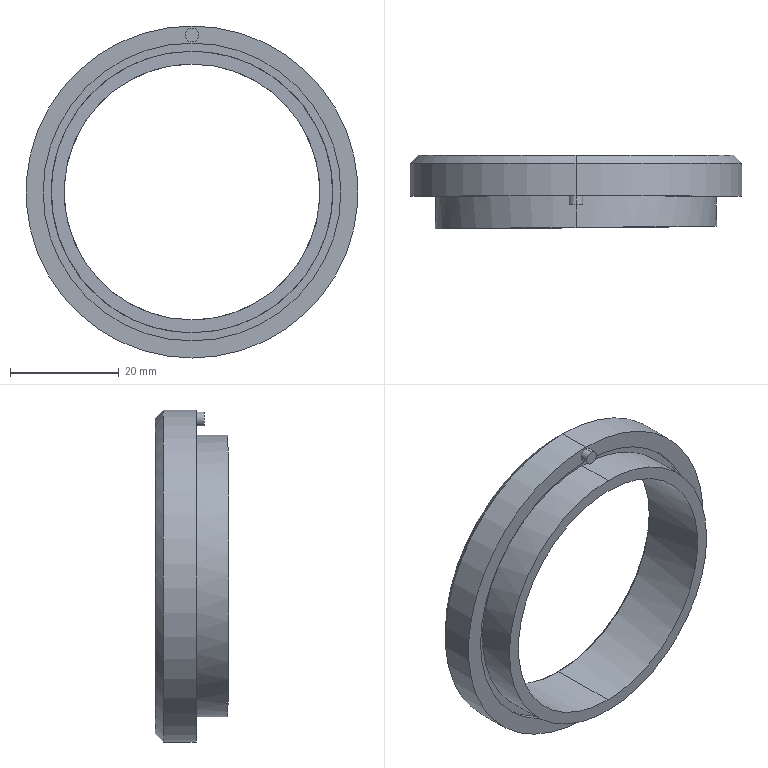Part | SolidWorks | features Chamfer 2, ICE 2, Revolution 1 | 1 solid | 19 faces | box 61 x 13.5 x 61 mm | volume 10536 mm3 | cylinder 10 | plane 5 | cone 4 | commonest cylinder face diameters 2.5 x2 47 x2 51.7 x2 54.7 x2 61 x2
STEP:
#1=CARTESIAN_POINT('',(0.,-1.5,27.6));
#2=VERTEX_POINT('',#1);
#3=CARTESIAN_POINT('',(0.,-1.5,30.1));
#4=VERTEX_POINT('',#3);
#5=CARTESIAN_POINT('',(0.,-1.5,28.85));
#6=DIRECTION('',(0.,-1.,0.));
#7=DIRECTION('',(0.,0.,-1.));
#8=AXIS2_PLACEMENT_3D('',#5,#6,#7);
#9=CIRCLE('',#8,1.25);
#10=EDGE_CURVE('',#2,#4,#9,.T.);
#11=ORIENTED_EDGE('',*,*,#10,.F.);
#12=CARTESIAN_POINT('',(0.,0.,27.6));
#13=VERTEX_POINT('',#12);
#14=CARTESIAN_POINT('',(0.,-1.5,27.6));
#15=DIRECTION('',(0.,1.,0.));
#16=VECTOR('',#15,1000.);
#17=LINE('',#14,#16);
#18=EDGE_CURVE('',#2,#13,#17,.T.);
#19=ORIENTED_EDGE('',*,*,#18,.T.);
#20=CARTESIAN_POINT('',(0.,0.,30.1));
#21=VERTEX_POINT('',#20);
#22=CARTESIAN_POINT('',(0.,0.,28.85));
#23=DIRECTION('',(0.,-1.,0.));
#24=DIRECTION('',(0.,0.,-1.));
#25=AXIS2_PLACEMENT_3D('',#22,#23,#24);
#26=CIRCLE('',#25,1.25);
#27=EDGE_CURVE('',#13,#21,#26,.T.);
#28=ORIENTED_EDGE('',*,*,#27,.T.);
#29=CARTESIAN_POINT('',(0.,-1.5,30.1));
#30=DIRECTION('',(0.,1.,0.));
#31=VECTOR('',#30,1000.);
#32=LINE('',#29,#31);
#33=EDGE_CURVE('',#4,#21,#32,.T.);
#34=ORIENTED_EDGE('',*,*,#33,.F.);
#35=EDGE_LOOP('',(#11,#19,#28,#34));
#36=FACE_OUTER_BOUND('',#35,.T.);
#37=CARTESIAN_POINT('',(0.,-1.5,28.85));
#38=DIRECTION('',(0.,1.,0.));
#39=DIRECTION('',(0.,0.,1.));
#40=AXIS2_PLACEMENT_3D('',#37,#38,#39);
#41=CYLINDRICAL_SURFACE('',#40,1.25);
#42=ADVANCED_FACE('',(#36),#41,.T.);
#43=CARTESIAN_POINT('',(0.,7.5,29.));
#44=VERTEX_POINT('',#43);
#45=CARTESIAN_POINT('',(0.,7.5,-29.));
#46=VERTEX_POINT('',#45);
#47=CARTESIAN_POINT('',(0.,7.5,0.));
#48=DIRECTION('',(0.,1.,0.));
#49=DIRECTION('',(0.,0.,1.));
#50=AXIS2_PLACEMENT_3D('',#47,#48,#49);
#51=CIRCLE('',#50,29.);
#52=EDGE_CURVE('',#44,#46,#51,.T.);
#53=ORIENTED_EDGE('',*,*,#52,.F.);
#54=CARTESIAN_POINT('',(0.,6.,30.5));
#55=VERTEX_POINT('',#54);
#56=CARTESIAN_POINT('',(0.,6.,30.5));
#57=DIRECTION('',(0.,-0.7071,0.7071));
#58=VECTOR('',#57,1000.);
#59=LINE('',#56,#58);
#60=EDGE_CURVE('',#44,#55,#59,.T.);
#61=ORIENTED_EDGE('',*,*,#60,.T.);
#62=CARTESIAN_POINT('',(0.,6.,-30.5));
#63=VERTEX_POINT('',#62);
#64=CARTESIAN_POINT('',(0.,6.,0.));
#65=DIRECTION('',(0.,-1.,0.));
#66=DIRECTION('',(0.,0.,1.));
#67=AXIS2_PLACEMENT_3D('',#64,#65,#66);
#68=CIRCLE('',#67,30.5);
#69=EDGE_CURVE('',#63,#55,#68,.T.);
#70=ORIENTED_EDGE('',*,*,#69,.F.);
#71=CARTESIAN_POINT('',(0.,6.,-30.5));
#72=DIRECTION('',(0.,-0.7071,-0.7071));
#73=VECTOR('',#72,1000.);
#74=LINE('',#71,#73);
#75=EDGE_CURVE('',#46,#63,#74,.T.);
#76=ORIENTED_EDGE('',*,*,#75,.F.);
#77=EDGE_LOOP('',(#53,#61,#70,#76));
#78=FACE_OUTER_BOUND('',#77,.T.);
#79=CARTESIAN_POINT('',(0.,6.,0.));
#80=DIRECTION('',(0.,-1.,0.));
#81=DIRECTION('',(0.,0.,-1.));
#82=AXIS2_PLACEMENT_3D('',#79,#80,#81);
#83=CONICAL_SURFACE('',#82,30.5,0.7854);
#84=ADVANCED_FACE('',(#78),#83,.T.);
#85=CARTESIAN_POINT('',(0.,7.,-23.5));
#86=VERTEX_POINT('',#85);
#87=CARTESIAN_POINT('',(0.,7.,23.5));
#88=VERTEX_POINT('',#87);
#89=CARTESIAN_POINT('',(0.,7.,0.));
#90=DIRECTION('',(0.,1.,0.));
#91=DIRECTION('',(0.,0.,1.));
#92=AXIS2_PLACEMENT_3D('',#89,#90,#91);
#93=CIRCLE('',#92,23.5);
#94=EDGE_CURVE('',#86,#88,#93,.T.);
#95=ORIENTED_EDGE('',*,*,#94,.F.);
#96=CARTESIAN_POINT('',(0.,7.5,-24.));
#97=VERTEX_POINT('',#96);
#98=CARTESIAN_POINT('',(0.,7.5,-24.));
#99=DIRECTION('',(0.,0.7071,-0.7071));
#100=VECTOR('',#99,1000.);
#101=LINE('',#98,#100);
#102=EDGE_CURVE('',#86,#97,#101,.T.);
#103=ORIENTED_EDGE('',*,*,#102,.T.);
#104=CARTESIAN_POINT('',(0.,7.5,24.));
#105=VERTEX_POINT('',#104);
#106=CARTESIAN_POINT('',(0.,7.5,0.));
#107=DIRECTION('',(0.,-1.,0.));
#108=DIRECTION('',(0.,0.,1.));
#109=AXIS2_PLACEMENT_3D('',#106,#107,#108);
#110=CIRCLE('',#109,24.);
#111=EDGE_CURVE('',#105,#97,#110,.T.);
#112=ORIENTED_EDGE('',*,*,#111,.F.);
#113=CARTESIAN_POINT('',(0.,7.5,24.));
#114=DIRECTION('',(0.,0.7071,0.7071));
#115=VECTOR('',#114,1000.);
#116=LINE('',#113,#115);
#117=EDGE_CURVE('',#88,#105,#116,.T.);
#118=ORIENTED_EDGE('',*,*,#117,.F.);
#119=EDGE_LOOP('',(#95,#103,#112,#118));
#120=FACE_OUTER_BOUND('',#119,.T.);
#121=CARTESIAN_POINT('',(0.,7.5,0.));
#122=DIRECTION('',(0.,1.,0.));
#123=DIRECTION('',(0.,0.,1.));
#124=AXIS2_PLACEMENT_3D('',#121,#122,#123);
#125=CONICAL_SURFACE('',#124,24.,0.7854);
#126=ADVANCED_FACE('',(#120),#125,.F.);
#127=CARTESIAN_POINT('',(0.,1.,-25.85));
#128=VERTEX_POINT('',#127);
#129=CARTESIAN_POINT('',(0.,1.,25.85));
#130=VERTEX_POINT('',#129);
#131=CARTESIAN_POINT('',(0.,1.,0.));
#132=DIRECTION('',(0.,-1.,0.));
#133=DIRECTION('',(0.,0.,-1.));
#134=AXIS2_PLACEMENT_3D('',#131,#132,#133);
#135=CIRCLE('',#134,25.85);
#136=EDGE_CURVE('',#128,#130,#135,.T.);
#137=ORIENTED_EDGE('',*,*,#136,.T.);
#138=CARTESIAN_POINT('',(0.,-5.774,25.85));
#139=VERTEX_POINT('',#138);
#140=CARTESIAN_POINT('',(0.,0.,25.85));
#141=DIRECTION('',(0.,-1.,0.));
#142=VECTOR('',#141,1000.);
#143=LINE('',#140,#142);
#144=EDGE_CURVE('',#130,#139,#143,.T.);
#145=ORIENTED_EDGE('',*,*,#144,.T.);
#146=CARTESIAN_POINT('',(0.,-5.774,-25.85));
#147=VERTEX_POINT('',#146);
#148=CARTESIAN_POINT('',(0.,-5.774,-25.85));
#149=CARTESIAN_POINT('',(51.7,-5.323,-25.85));
#150=CARTESIAN_POINT('',(51.7,-5.323,25.85));
#151=CARTESIAN_POINT('',(0.,-5.774,25.85));
#152=(BOUNDED_CURVE()B_SPLINE_CURVE(3,(#148,#149,#150,#151),.UNSPECIFIED.,.F.,.F.)B_SPLINE_CURVE_WITH_KNOTS((4,4),(1.571,4.712),.UNSPECIFIED.)CURVE()GEOMETRIC_REPRESENTATION_ITEM()RATIONAL_B_SPLINE_CURVE((1.,0.3333,0.3333,1.))REPRESENTATION_ITEM(''));
#153=EDGE_CURVE('',#147,#139,#152,.T.);
#154=ORIENTED_EDGE('',*,*,#153,.F.);
#155=CARTESIAN_POINT('',(0.,0.,-25.85));
#156=DIRECTION('',(0.,-1.,0.));
#157=VECTOR('',#156,1000.);
#158=LINE('',#155,#157);
#159=EDGE_CURVE('',#128,#147,#158,.T.);
#160=ORIENTED_EDGE('',*,*,#159,.F.);
#161=EDGE_LOOP('',(#137,#145,#154,#160));
#162=FACE_OUTER_BOUND('',#161,.T.);
#163=CARTESIAN_POINT('',(0.,0.,0.));
#164=DIRECTION('',(0.,-1.,0.));
#165=DIRECTION('',(0.,0.,-1.));
#166=AXIS2_PLACEMENT_3D('',#163,#164,#165);
#167=CYLINDRICAL_SURFACE('',#166,25.85);
#168=ADVANCED_FACE('',(#162),#167,.T.);
#169=CARTESIAN_POINT('',(0.,1.,27.35));
#170=VERTEX_POINT('',#169);
#171=CARTESIAN_POINT('',(0.,1.,-27.35));
#172=VERTEX_POINT('',#171);
#173=CARTESIAN_POINT('',(0.,1.,0.));
#174=DIRECTION('',(0.,-1.,0.));
#175=DIRECTION('',(0.,0.,-1.));
#176=AXIS2_PLACEMENT_3D('',#173,#174,#175);
#177=CIRCLE('',#176,27.35);
#178=EDGE_CURVE('',#170,#172,#177,.T.);
#179=ORIENTED_EDGE('',*,*,#178,.F.);
#180=CARTESIAN_POINT('',(0.,0.,27.35));
#181=VERTEX_POINT('',#180);
#182=CARTESIAN_POINT('',(0.,0.,27.35));
#183=DIRECTION('',(0.,-1.,0.));
#184=VECTOR('',#183,1000.);
#185=LINE('',#182,#184);
#186=EDGE_CURVE('',#170,#181,#185,.T.);
#187=ORIENTED_EDGE('',*,*,#186,.T.);
#188=CARTESIAN_POINT('',(0.,0.,-27.35));
#189=VERTEX_POINT('',#188);
#190=CARTESIAN_POINT('',(0.,0.,0.));
#191=DIRECTION('',(0.,-1.,0.));
#192=DIRECTION('',(0.,0.,-1.));
#193=AXIS2_PLACEMENT_3D('',#190,#191,#192);
#194=CIRCLE('',#193,27.35);
#195=EDGE_CURVE('',#181,#189,#194,.T.);
#196=ORIENTED_EDGE('',*,*,#195,.T.);
#197=CARTESIAN_POINT('',(0.,0.,-27.35));
#198=DIRECTION('',(0.,-1.,0.));
#199=VECTOR('',#198,1000.);
#200=LINE('',#197,#199);
#201=EDGE_CURVE('',#172,#189,#200,.T.);
#202=ORIENTED_EDGE('',*,*,#201,.F.);
#203=EDGE_LOOP('',(#179,#187,#196,#202));
#204=FACE_OUTER_BOUND('',#203,.T.);
#205=CARTESIAN_POINT('',(0.,0.,0.));
#206=DIRECTION('',(0.,-1.,0.));
#207=DIRECTION('',(0.,0.,-1.));
#208=AXIS2_PLACEMENT_3D('',#205,#206,#207);
#209=CYLINDRICAL_SURFACE('',#208,27.35);
#210=ADVANCED_FACE('',(#204),#209,.F.);
#211=ORIENTED_EDGE('',*,*,#69,.T.);
#212=CARTESIAN_POINT('',(0.,0.,30.5));
#213=VERTEX_POINT('',#212);
#214=CARTESIAN_POINT('',(0.,0.,30.5));
#215=DIRECTION('',(0.,-1.,0.));
#216=VECTOR('',#215,1000.);
#217=LINE('',#214,#216);
#218=EDGE_CURVE('',#55,#213,#217,.T.);
#219=ORIENTED_EDGE('',*,*,#218,.T.);
#220=CARTESIAN_POINT('',(0.,0.,-30.5));
#221=VERTEX_POINT('',#220);
#222=CARTESIAN_POINT('',(0.,0.,0.));
#223=DIRECTION('',(0.,-1.,0.));
#224=DIRECTION('',(0.,0.,-1.));
#225=AXIS2_PLACEMENT_3D('',#222,#223,#224);
#226=CIRCLE('',#225,30.5);
#227=EDGE_CURVE('',#221,#213,#226,.T.);
#228=ORIENTED_EDGE('',*,*,#227,.F.);
#229=CARTESIAN_POINT('',(0.,0.,-30.5));
#230=DIRECTION('',(0.,-1.,0.));
#231=VECTOR('',#230,1000.);
#232=LINE('',#229,#231);
#233=EDGE_CURVE('',#63,#221,#232,.T.);
#234=ORIENTED_EDGE('',*,*,#233,.F.);
#235=EDGE_LOOP('',(#211,#219,#228,#234));
#236=FACE_OUTER_BOUND('',#235,.T.);
#237=CARTESIAN_POINT('',(0.,0.,0.));
#238=DIRECTION('',(0.,-1.,0.));
#239=DIRECTION('',(0.,0.,-1.));
#240=AXIS2_PLACEMENT_3D('',#237,#238,#239);
#241=CYLINDRICAL_SURFACE('',#240,30.5);
#242=ADVANCED_FACE('',(#236),#241,.T.);
#243=ORIENTED_EDGE('',*,*,#94,.T.);
#244=CARTESIAN_POINT('',(0.,-5.774,23.5));
#245=VERTEX_POINT('',#244);
#246=CARTESIAN_POINT('',(0.,0.,23.5));
#247=DIRECTION('',(0.,-1.,0.));
#248=VECTOR('',#247,1000.);
#249=LINE('',#246,#248);
#250=EDGE_CURVE('',#88,#245,#249,.T.);
#251=ORIENTED_EDGE('',*,*,#250,.T.);
#252=CARTESIAN_POINT('',(0.,-5.774,-23.5));
#253=VERTEX_POINT('',#252);
#254=CARTESIAN_POINT('',(0.,-5.774,-23.5));
#255=CARTESIAN_POINT('',(-47.,-6.185,-23.5));
#256=CARTESIAN_POINT('',(-47.,-6.185,23.5));
#257=CARTESIAN_POINT('',(0.,-5.774,23.5));
#258=(BOUNDED_CURVE()B_SPLINE_CURVE(3,(#254,#255,#256,#257),.UNSPECIFIED.,.F.,.F.)B_SPLINE_CURVE_WITH_KNOTS((4,4),(4.712,7.854),.UNSPECIFIED.)CURVE()GEOMETRIC_REPRESENTATION_ITEM()RATIONAL_B_SPLINE_CURVE((1.,0.3333,0.3333,1.))REPRESENTATION_ITEM(''));
#259=EDGE_CURVE('',#253,#245,#258,.T.);
#260=ORIENTED_EDGE('',*,*,#259,.F.);
#261=CARTESIAN_POINT('',(0.,0.,-23.5));
#262=DIRECTION('',(0.,-1.,0.));
#263=VECTOR('',#262,1000.);
#264=LINE('',#261,#263);
#265=EDGE_CURVE('',#86,#253,#264,.T.);
#266=ORIENTED_EDGE('',*,*,#265,.F.);
#267=EDGE_LOOP('',(#243,#251,#260,#266));
#268=FACE_OUTER_BOUND('',#267,.T.);
#269=CARTESIAN_POINT('',(0.,0.,0.));
#270=DIRECTION('',(0.,-1.,0.));
#271=DIRECTION('',(0.,0.,-1.));
#272=AXIS2_PLACEMENT_3D('',#269,#270,#271);
#273=CYLINDRICAL_SURFACE('',#272,23.5);
#274=ADVANCED_FACE('',(#268),#273,.F.);
#275=ORIENTED_EDGE('',*,*,#250,.F.);
#276=CARTESIAN_POINT('',(0.,7.,0.));
#277=DIRECTION('',(0.,1.,0.));
#278=DIRECTION('',(0.,0.,1.));
#279=AXIS2_PLACEMENT_3D('',#276,#277,#278);
#280=CIRCLE('',#279,23.5);
#281=EDGE_CURVE('',#88,#86,#280,.T.);
#282=ORIENTED_EDGE('',*,*,#281,.T.);
#283=ORIENTED_EDGE('',*,*,#265,.T.);
#284=CARTESIAN_POINT('',(0.,-5.774,23.5));
#285=CARTESIAN_POINT('',(47.,-5.364,23.5));
#286=CARTESIAN_POINT('',(47.,-5.364,-23.5));
#287=CARTESIAN_POINT('',(0.,-5.774,-23.5));
#288=(BOUNDED_CURVE()B_SPLINE_CURVE(3,(#284,#285,#286,#287),.UNSPECIFIED.,.F.,.F.)B_SPLINE_CURVE_WITH_KNOTS((4,4),(1.571,4.712),.UNSPECIFIED.)CURVE()GEOMETRIC_REPRESENTATION_ITEM()RATIONAL_B_SPLINE_CURVE((1.,0.3333,0.3333,1.))REPRESENTATION_ITEM(''));
#289=EDGE_CURVE('',#245,#253,#288,.T.);
#290=ORIENTED_EDGE('',*,*,#289,.F.);
#291=EDGE_LOOP('',(#275,#282,#283,#290));
#292=FACE_OUTER_BOUND('',#291,.T.);
#293=CARTESIAN_POINT('',(0.,0.,0.));
#294=DIRECTION('',(0.,-1.,0.));
#295=DIRECTION('',(0.,0.,-1.));
#296=AXIS2_PLACEMENT_3D('',#293,#294,#295);
#297=CYLINDRICAL_SURFACE('',#296,23.5);
#298=ADVANCED_FACE('',(#292),#297,.F.);
#299=CARTESIAN_POINT('',(0.,7.5,0.));
#300=DIRECTION('',(0.,1.,0.));
#301=DIRECTION('',(0.,0.,1.));
#302=AXIS2_PLACEMENT_3D('',#299,#300,#301);
#303=CIRCLE('',#302,29.);
#304=EDGE_CURVE('',#46,#44,#303,.T.);
#305=ORIENTED_EDGE('',*,*,#304,.T.);
#306=ORIENTED_EDGE('',*,*,#52,.T.);
#307=EDGE_LOOP('',(#305,#306));
#308=FACE_OUTER_BOUND('',#307,.T.);
#309=ORIENTED_EDGE('',*,*,#111,.T.);
#310=CARTESIAN_POINT('',(0.,7.5,0.));
#311=DIRECTION('',(0.,-1.,0.));
#312=DIRECTION('',(0.,0.,1.));
#313=AXIS2_PLACEMENT_3D('',#310,#311,#312);
#314=CIRCLE('',#313,24.);
#315=EDGE_CURVE('',#97,#105,#314,.T.);
#316=ORIENTED_EDGE('',*,*,#315,.T.);
#317=EDGE_LOOP('',(#309,#316));
#318=FACE_BOUND('',#317,.T.);
#319=CARTESIAN_POINT('',(30.5,7.5,0.));
#320=DIRECTION('',(0.,1.,0.));
#321=DIRECTION('',(0.,0.,1.));
#322=AXIS2_PLACEMENT_3D('',#319,#320,#321);
#323=PLANE('',#322);
#324=ADVANCED_FACE('',(#308,#318),#323,.T.);
#325=ORIENTED_EDGE('',*,*,#218,.F.);
#326=CARTESIAN_POINT('',(0.,6.,0.));
#327=DIRECTION('',(0.,-1.,0.));
#328=DIRECTION('',(0.,0.,1.));
#329=AXIS2_PLACEMENT_3D('',#326,#327,#328);
#330=CIRCLE('',#329,30.5);
#331=EDGE_CURVE('',#55,#63,#330,.T.);
#332=ORIENTED_EDGE('',*,*,#331,.T.);
#333=ORIENTED_EDGE('',*,*,#233,.T.);
#334=CARTESIAN_POINT('',(0.,0.,0.));
#335=DIRECTION('',(0.,-1.,0.));
#336=DIRECTION('',(0.,0.,-1.));
#337=AXIS2_PLACEMENT_3D('',#334,#335,#336);
#338=CIRCLE('',#337,30.5);
#339=EDGE_CURVE('',#213,#221,#338,.T.);
#340=ORIENTED_EDGE('',*,*,#339,.F.);
#341=EDGE_LOOP('',(#325,#332,#333,#340));
#342=FACE_OUTER_BOUND('',#341,.T.);
#343=CARTESIAN_POINT('',(0.,0.,0.));
#344=DIRECTION('',(0.,-1.,0.));
#345=DIRECTION('',(0.,0.,-1.));
#346=AXIS2_PLACEMENT_3D('',#343,#344,#345);
#347=CYLINDRICAL_SURFACE('',#346,30.5);
#348=ADVANCED_FACE('',(#342),#347,.T.);
#349=CARTESIAN_POINT('',(0.,0.,28.85));
#350=DIRECTION('',(0.,-1.,0.));
#351=DIRECTION('',(0.,0.,-1.));
#352=AXIS2_PLACEMENT_3D('',#349,#350,#351);
#353=CIRCLE('',#352,1.25);
#354=EDGE_CURVE('',#21,#13,#353,.T.);
#355=ORIENTED_EDGE('',*,*,#354,.F.);
#356=ORIENTED_EDGE('',*,*,#27,.F.);
#357=EDGE_LOOP('',(#355,#356));
#358=FACE_BOUND('',#357,.T.);
#359=ORIENTED_EDGE('',*,*,#227,.T.);
#360=ORIENTED_EDGE('',*,*,#339,.T.);
#361=EDGE_LOOP('',(#359,#360));
#362=FACE_OUTER_BOUND('',#361,.T.);
#363=CARTESIAN_POINT('',(0.,0.,0.));
#364=DIRECTION('',(0.,-1.,0.));
#365=DIRECTION('',(0.,0.,-1.));
#366=AXIS2_PLACEMENT_3D('',#363,#364,#365);
#367=CIRCLE('',#366,27.35);
#368=EDGE_CURVE('',#189,#181,#367,.T.);
#369=ORIENTED_EDGE('',*,*,#368,.F.);
#370=ORIENTED_EDGE('',*,*,#195,.F.);
#371=EDGE_LOOP('',(#369,#370));
#372=FACE_BOUND('',#371,.T.);
#373=CARTESIAN_POINT('',(30.5,0.,0.));
#374=DIRECTION('',(0.,-1.,0.));
#375=DIRECTION('',(0.,0.,-1.));
#376=AXIS2_PLACEMENT_3D('',#373,#374,#375);
#377=PLANE('',#376);
#378=ADVANCED_FACE('',(#358,#362,#372),#377,.T.);
#379=ORIENTED_EDGE('',*,*,#186,.F.);
#380=CARTESIAN_POINT('',(0.,1.,0.));
#381=DIRECTION('',(0.,-1.,0.));
#382=DIRECTION('',(0.,0.,-1.));
#383=AXIS2_PLACEMENT_3D('',#380,#381,#382);
#384=CIRCLE('',#383,27.35);
#385=EDGE_CURVE('',#172,#170,#384,.T.);
#386=ORIENTED_EDGE('',*,*,#385,.F.);
#387=ORIENTED_EDGE('',*,*,#201,.T.);
#388=ORIENTED_EDGE('',*,*,#368,.T.);
#389=EDGE_LOOP('',(#379,#386,#387,#388));
#390=FACE_OUTER_BOUND('',#389,.T.);
#391=CARTESIAN_POINT('',(0.,0.,0.));
#392=DIRECTION('',(0.,-1.,0.));
#393=DIRECTION('',(0.,0.,-1.));
#394=AXIS2_PLACEMENT_3D('',#391,#392,#393);
#395=CYLINDRICAL_SURFACE('',#394,27.35);
#396=ADVANCED_FACE('',(#390),#395,.F.);
#397=ORIENTED_EDGE('',*,*,#385,.T.);
#398=ORIENTED_EDGE('',*,*,#178,.T.);
#399=EDGE_LOOP('',(#397,#398));
#400=FACE_OUTER_BOUND('',#399,.T.);
#401=ORIENTED_EDGE('',*,*,#136,.F.);
#402=CARTESIAN_POINT('',(0.,1.,0.));
#403=DIRECTION('',(0.,-1.,0.));
#404=DIRECTION('',(0.,0.,-1.));
#405=AXIS2_PLACEMENT_3D('',#402,#403,#404);
#406=CIRCLE('',#405,25.85);
#407=EDGE_CURVE('',#130,#128,#406,.T.);
#408=ORIENTED_EDGE('',*,*,#407,.F.);
#409=EDGE_LOOP('',(#401,#408));
#410=FACE_BOUND('',#409,.T.);
#411=CARTESIAN_POINT('',(27.35,1.,0.));
#412=DIRECTION('',(0.,-1.,0.));
#413=DIRECTION('',(0.,0.,-1.));
#414=AXIS2_PLACEMENT_3D('',#411,#412,#413);
#415=PLANE('',#414);
#416=ADVANCED_FACE('',(#400,#410),#415,.T.);
#417=ORIENTED_EDGE('',*,*,#144,.F.);
#418=ORIENTED_EDGE('',*,*,#407,.T.);
#419=ORIENTED_EDGE('',*,*,#159,.T.);
#420=CARTESIAN_POINT('',(0.,-5.774,25.85));
#421=CARTESIAN_POINT('',(-51.7,-6.226,25.85));
#422=CARTESIAN_POINT('',(-51.7,-6.226,-25.85));
#423=CARTESIAN_POINT('',(0.,-5.774,-25.85));
#424=(BOUNDED_CURVE()B_SPLINE_CURVE(3,(#420,#421,#422,#423),.UNSPECIFIED.,.F.,.F.)B_SPLINE_CURVE_WITH_KNOTS((4,4),(4.712,7.854),.UNSPECIFIED.)CURVE()GEOMETRIC_REPRESENTATION_ITEM()RATIONAL_B_SPLINE_CURVE((1.,0.3333,0.3333,1.))REPRESENTATION_ITEM(''));
#425=EDGE_CURVE('',#139,#147,#424,.T.);
#426=ORIENTED_EDGE('',*,*,#425,.F.);
#427=EDGE_LOOP('',(#417,#418,#419,#426));
#428=FACE_OUTER_BOUND('',#427,.T.);
#429=CARTESIAN_POINT('',(0.,0.,0.));
#430=DIRECTION('',(0.,-1.,0.));
#431=DIRECTION('',(0.,0.,-1.));
#432=AXIS2_PLACEMENT_3D('',#429,#430,#431);
#433=CYLINDRICAL_SURFACE('',#432,25.85);
#434=ADVANCED_FACE('',(#428),#433,.T.);
#435=ORIENTED_EDGE('',*,*,#259,.T.);
#436=ORIENTED_EDGE('',*,*,#289,.T.);
#437=EDGE_LOOP('',(#435,#436));
#438=FACE_BOUND('',#437,.T.);
#439=ORIENTED_EDGE('',*,*,#153,.T.);
#440=ORIENTED_EDGE('',*,*,#425,.T.);
#441=EDGE_LOOP('',(#439,#440));
#442=FACE_OUTER_BOUND('',#441,.T.);
#443=CARTESIAN_POINT('',(-25.85,-6.,-30.5));
#444=DIRECTION('',(-0.008727,1.,0.));
#445=DIRECTION('',(-1.,-0.008727,0.));
#446=AXIS2_PLACEMENT_3D('',#443,#444,#445);
#447=PLANE('',#446);
#448=ADVANCED_FACE('',(#438,#442),#447,.F.);
#449=ORIENTED_EDGE('',*,*,#102,.F.);
#450=ORIENTED_EDGE('',*,*,#281,.F.);
#451=ORIENTED_EDGE('',*,*,#117,.T.);
#452=ORIENTED_EDGE('',*,*,#315,.F.);
#453=EDGE_LOOP('',(#449,#450,#451,#452));
#454=FACE_OUTER_BOUND('',#453,.T.);
#455=CARTESIAN_POINT('',(0.,7.5,0.));
#456=DIRECTION('',(0.,1.,0.));
#457=DIRECTION('',(0.,0.,1.));
#458=AXIS2_PLACEMENT_3D('',#455,#456,#457);
#459=CONICAL_SURFACE('',#458,24.,0.7854);
#460=ADVANCED_FACE('',(#454),#459,.F.);
#461=ORIENTED_EDGE('',*,*,#60,.F.);
#462=ORIENTED_EDGE('',*,*,#304,.F.);
#463=ORIENTED_EDGE('',*,*,#75,.T.);
#464=ORIENTED_EDGE('',*,*,#331,.F.);
#465=EDGE_LOOP('',(#461,#462,#463,#464));
#466=FACE_OUTER_BOUND('',#465,.T.);
#467=CARTESIAN_POINT('',(0.,6.,0.));
#468=DIRECTION('',(0.,-1.,0.));
#469=DIRECTION('',(0.,0.,-1.));
#470=AXIS2_PLACEMENT_3D('',#467,#468,#469);
#471=CONICAL_SURFACE('',#470,30.5,0.7854);
#472=ADVANCED_FACE('',(#466),#471,.T.);
#473=ORIENTED_EDGE('',*,*,#18,.F.);
#474=CARTESIAN_POINT('',(0.,-1.5,28.85));
#475=DIRECTION('',(0.,-1.,0.));
#476=DIRECTION('',(0.,0.,-1.));
#477=AXIS2_PLACEMENT_3D('',#474,#475,#476);
#478=CIRCLE('',#477,1.25);
#479=EDGE_CURVE('',#4,#2,#478,.T.);
#480=ORIENTED_EDGE('',*,*,#479,.F.);
#481=ORIENTED_EDGE('',*,*,#33,.T.);
#482=ORIENTED_EDGE('',*,*,#354,.T.);
#483=EDGE_LOOP('',(#473,#480,#481,#482));
#484=FACE_OUTER_BOUND('',#483,.T.);
#485=CARTESIAN_POINT('',(0.,-1.5,28.85));
#486=DIRECTION('',(0.,1.,0.));
#487=DIRECTION('',(0.,0.,1.));
#488=AXIS2_PLACEMENT_3D('',#485,#486,#487);
#489=CYLINDRICAL_SURFACE('',#488,1.25);
#490=ADVANCED_FACE('',(#484),#489,.T.);
#491=ORIENTED_EDGE('',*,*,#479,.T.);
#492=ORIENTED_EDGE('',*,*,#10,.T.);
#493=EDGE_LOOP('',(#491,#492));
#494=FACE_OUTER_BOUND('',#493,.T.);
#495=CARTESIAN_POINT('',(0.,-1.5,28.85));
#496=DIRECTION('',(0.,-1.,0.));
#497=DIRECTION('',(0.,0.,-1.));
#498=AXIS2_PLACEMENT_3D('',#495,#496,#497);
#499=PLANE('',#498);
#500=ADVANCED_FACE('',(#494),#499,.T.);
#501=CLOSED_SHELL('',(#42,#84,#126,#168,#210,#242,#274,#298,#324,#348,#378,#396,#416,#434,#448,#460,#472,#490,#500));
#502=MANIFOLD_SOLID_BREP('',#501);
#503=CARTESIAN_POINT('',(0.,0.,0.));
#504=DIRECTION('',(0.,0.,1.));
#505=DIRECTION('',(1.,0.,0.));
#506=AXIS2_PLACEMENT_3D('',#503,#504,#505);
#507=(LENGTH_UNIT()NAMED_UNIT(*)SI_UNIT(.MILLI.,.METRE.));
#508=UNCERTAINTY_MEASURE_WITH_UNIT(LENGTH_MEASURE(0.00001),#507,'','');
#509=(NAMED_UNIT(*)PLANE_ANGLE_UNIT()SI_UNIT($,.RADIAN.));
#510=(NAMED_UNIT(*)SI_UNIT($,.STERADIAN.)SOLID_ANGLE_UNIT());
#511=(GEOMETRIC_REPRESENTATION_CONTEXT(3)GLOBAL_UNCERTAINTY_ASSIGNED_CONTEXT((#508))GLOBAL_UNIT_ASSIGNED_CONTEXT((#507,#509,#510))REPRESENTATION_CONTEXT('',''));
#512=ADVANCED_BREP_SHAPE_REPRESENTATION('',(#502,#506),#511);